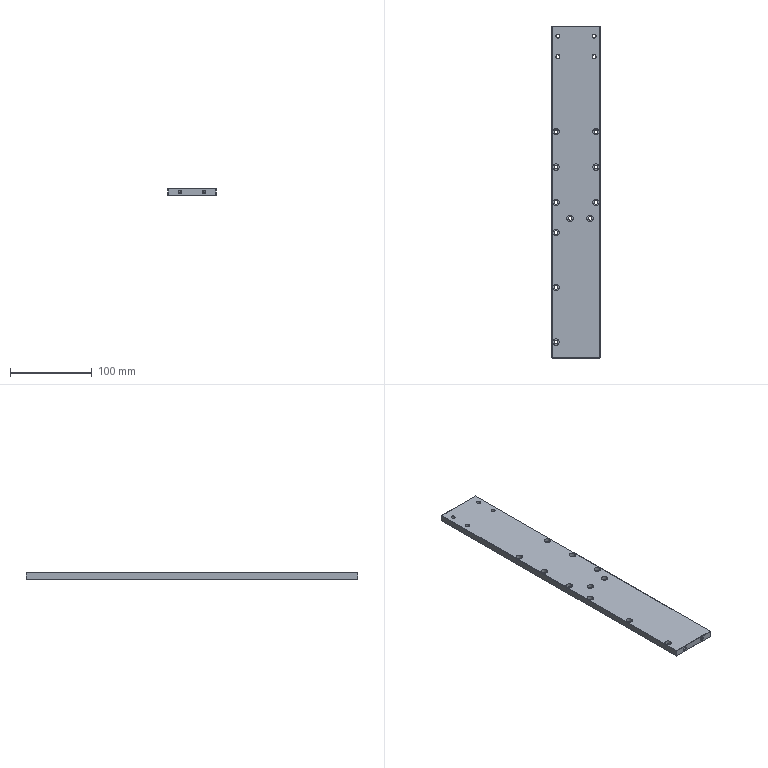Part | NX | 1 solid | 105 faces | box 59 x 406.5 x 8 mm | volume 188006 mm3 | cylinder 60 | plane 29 | cone 16 | commonest cylinder face diameters 4.5 x30 8 x22 3.3 x8